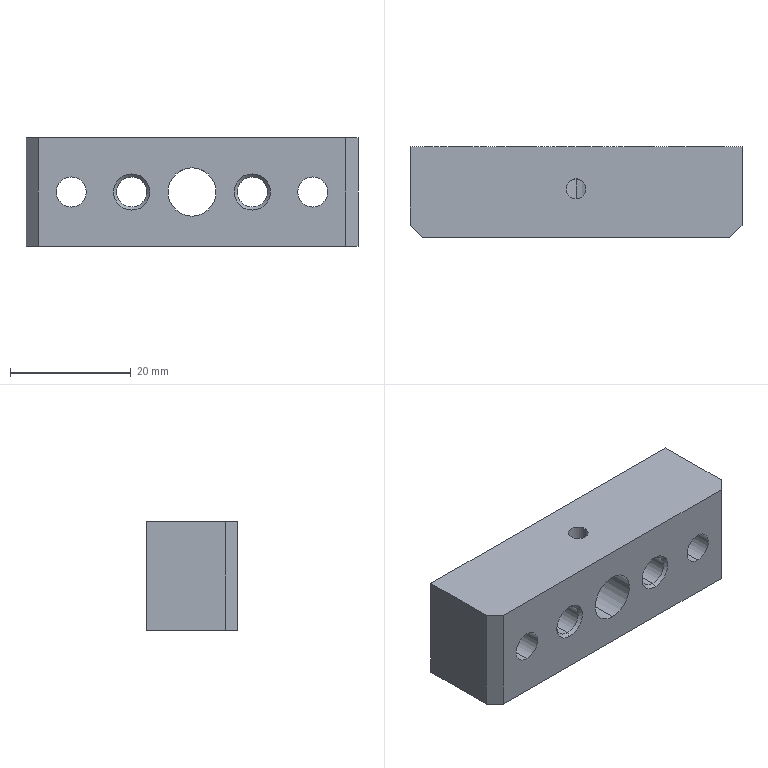Part | SolidWorks | features ICE 9, Chamfer 3, 3DProfileFeature 2, HoleWzd 2, Extrusion 1 | 1 solid | 38 faces | box 55 x 15 x 18 mm | volume 12154 mm3 | cylinder 16 | cone 12 | plane 10 | commonest cylinder face diameters 5 x8 8 x6 3.3 x2
STEP:
#1=CARTESIAN_POINT('',(-20.,14.,-4.));
#2=VERTEX_POINT('',#1);
#3=CARTESIAN_POINT('',(-20.,14.,4.));
#4=VERTEX_POINT('',#3);
#5=CARTESIAN_POINT('',(-20.,14.,0.));
#6=DIRECTION('',(0.,1.,0.));
#7=DIRECTION('',(0.,0.,-1.));
#8=AXIS2_PLACEMENT_3D('',#5,#6,#7);
#9=CIRCLE('',#8,4.);
#10=EDGE_CURVE('',#2,#4,#9,.T.);
#11=ORIENTED_EDGE('',*,*,#10,.F.);
#12=CARTESIAN_POINT('',(-20.,15.,-5.));
#13=VERTEX_POINT('',#12);
#14=CARTESIAN_POINT('',(-20.,14.,-4.));
#15=DIRECTION('',(0.,0.7071,-0.7071));
#16=VECTOR('',#15,1000.);
#17=LINE('',#14,#16);
#18=EDGE_CURVE('',#2,#13,#17,.T.);
#19=ORIENTED_EDGE('',*,*,#18,.T.);
#20=CARTESIAN_POINT('',(-20.,15.,5.));
#21=VERTEX_POINT('',#20);
#22=CARTESIAN_POINT('',(-20.,15.,0.));
#23=DIRECTION('',(0.,-1.,0.));
#24=DIRECTION('',(0.,0.,-1.));
#25=AXIS2_PLACEMENT_3D('',#22,#23,#24);
#26=CIRCLE('',#25,5.);
#27=EDGE_CURVE('',#21,#13,#26,.T.);
#28=ORIENTED_EDGE('',*,*,#27,.F.);
#29=CARTESIAN_POINT('',(-20.,14.,4.));
#30=DIRECTION('',(0.,0.7071,0.7071));
#31=VECTOR('',#30,1000.);
#32=LINE('',#29,#31);
#33=EDGE_CURVE('',#4,#21,#32,.T.);
#34=ORIENTED_EDGE('',*,*,#33,.F.);
#35=EDGE_LOOP('',(#11,#19,#28,#34));
#36=FACE_OUTER_BOUND('',#35,.T.);
#37=CARTESIAN_POINT('',(-20.,14.,0.));
#38=DIRECTION('',(0.,1.,0.));
#39=DIRECTION('',(0.,0.,1.));
#40=AXIS2_PLACEMENT_3D('',#37,#38,#39);
#41=CONICAL_SURFACE('',#40,4.,0.7854);
#42=ADVANCED_FACE('',(#36),#41,.F.);
#43=CARTESIAN_POINT('',(20.,14.,-4.));
#44=VERTEX_POINT('',#43);
#45=CARTESIAN_POINT('',(20.,14.,4.));
#46=VERTEX_POINT('',#45);
#47=CARTESIAN_POINT('',(20.,14.,0.));
#48=DIRECTION('',(0.,1.,0.));
#49=DIRECTION('',(0.,0.,-1.));
#50=AXIS2_PLACEMENT_3D('',#47,#48,#49);
#51=CIRCLE('',#50,4.);
#52=EDGE_CURVE('',#44,#46,#51,.T.);
#53=ORIENTED_EDGE('',*,*,#52,.F.);
#54=CARTESIAN_POINT('',(20.,15.,-5.));
#55=VERTEX_POINT('',#54);
#56=CARTESIAN_POINT('',(20.,14.,-4.));
#57=DIRECTION('',(0.,0.7071,-0.7071));
#58=VECTOR('',#57,1000.);
#59=LINE('',#56,#58);
#60=EDGE_CURVE('',#44,#55,#59,.T.);
#61=ORIENTED_EDGE('',*,*,#60,.T.);
#62=CARTESIAN_POINT('',(20.,15.,5.));
#63=VERTEX_POINT('',#62);
#64=CARTESIAN_POINT('',(20.,15.,0.));
#65=DIRECTION('',(0.,-1.,0.));
#66=DIRECTION('',(0.,0.,-1.));
#67=AXIS2_PLACEMENT_3D('',#64,#65,#66);
#68=CIRCLE('',#67,5.);
#69=EDGE_CURVE('',#63,#55,#68,.T.);
#70=ORIENTED_EDGE('',*,*,#69,.F.);
#71=CARTESIAN_POINT('',(20.,14.,4.));
#72=DIRECTION('',(0.,0.7071,0.7071));
#73=VECTOR('',#72,1000.);
#74=LINE('',#71,#73);
#75=EDGE_CURVE('',#46,#63,#74,.T.);
#76=ORIENTED_EDGE('',*,*,#75,.F.);
#77=EDGE_LOOP('',(#53,#61,#70,#76));
#78=FACE_OUTER_BOUND('',#77,.T.);
#79=CARTESIAN_POINT('',(20.,14.,0.));
#80=DIRECTION('',(0.,1.,0.));
#81=DIRECTION('',(0.,0.,1.));
#82=AXIS2_PLACEMENT_3D('',#79,#80,#81);
#83=CONICAL_SURFACE('',#82,4.,0.7854);
#84=ADVANCED_FACE('',(#78),#83,.F.);
#85=CARTESIAN_POINT('',(-10.,14.5,-2.5));
#86=VERTEX_POINT('',#85);
#87=CARTESIAN_POINT('',(-10.,14.5,2.5));
#88=VERTEX_POINT('',#87);
#89=CARTESIAN_POINT('',(-10.,14.5,0.));
#90=DIRECTION('',(0.,1.,0.));
#91=DIRECTION('',(0.,0.,-1.));
#92=AXIS2_PLACEMENT_3D('',#89,#90,#91);
#93=CIRCLE('',#92,2.5);
#94=EDGE_CURVE('',#86,#88,#93,.T.);
#95=ORIENTED_EDGE('',*,*,#94,.F.);
#96=CARTESIAN_POINT('',(-10.,15.,-3.));
#97=VERTEX_POINT('',#96);
#98=CARTESIAN_POINT('',(-10.,14.5,-2.5));
#99=DIRECTION('',(0.,0.7071,-0.7071));
#100=VECTOR('',#99,1000.);
#101=LINE('',#98,#100);
#102=EDGE_CURVE('',#86,#97,#101,.T.);
#103=ORIENTED_EDGE('',*,*,#102,.T.);
#104=CARTESIAN_POINT('',(-10.,15.,3.));
#105=VERTEX_POINT('',#104);
#106=CARTESIAN_POINT('',(-10.,15.,0.));
#107=DIRECTION('',(0.,-1.,0.));
#108=DIRECTION('',(0.,0.,-1.));
#109=AXIS2_PLACEMENT_3D('',#106,#107,#108);
#110=CIRCLE('',#109,3.);
#111=EDGE_CURVE('',#105,#97,#110,.T.);
#112=ORIENTED_EDGE('',*,*,#111,.F.);
#113=CARTESIAN_POINT('',(-10.,14.5,2.5));
#114=DIRECTION('',(0.,0.7071,0.7071));
#115=VECTOR('',#114,1000.);
#116=LINE('',#113,#115);
#117=EDGE_CURVE('',#88,#105,#116,.T.);
#118=ORIENTED_EDGE('',*,*,#117,.F.);
#119=EDGE_LOOP('',(#95,#103,#112,#118));
#120=FACE_OUTER_BOUND('',#119,.T.);
#121=CARTESIAN_POINT('',(-10.,14.5,0.));
#122=DIRECTION('',(0.,1.,0.));
#123=DIRECTION('',(0.,0.,1.));
#124=AXIS2_PLACEMENT_3D('',#121,#122,#123);
#125=CONICAL_SURFACE('',#124,2.5,0.7854);
#126=ADVANCED_FACE('',(#120),#125,.F.);
#127=CARTESIAN_POINT('',(10.,14.5,-2.5));
#128=VERTEX_POINT('',#127);
#129=CARTESIAN_POINT('',(10.,14.5,2.5));
#130=VERTEX_POINT('',#129);
#131=CARTESIAN_POINT('',(10.,14.5,0.));
#132=DIRECTION('',(0.,1.,0.));
#133=DIRECTION('',(0.,0.,-1.));
#134=AXIS2_PLACEMENT_3D('',#131,#132,#133);
#135=CIRCLE('',#134,2.5);
#136=EDGE_CURVE('',#128,#130,#135,.T.);
#137=ORIENTED_EDGE('',*,*,#136,.F.);
#138=CARTESIAN_POINT('',(10.,15.,-3.));
#139=VERTEX_POINT('',#138);
#140=CARTESIAN_POINT('',(10.,14.5,-2.5));
#141=DIRECTION('',(0.,0.7071,-0.7071));
#142=VECTOR('',#141,1000.);
#143=LINE('',#140,#142);
#144=EDGE_CURVE('',#128,#139,#143,.T.);
#145=ORIENTED_EDGE('',*,*,#144,.T.);
#146=CARTESIAN_POINT('',(10.,15.,3.));
#147=VERTEX_POINT('',#146);
#148=CARTESIAN_POINT('',(10.,15.,0.));
#149=DIRECTION('',(0.,-1.,0.));
#150=DIRECTION('',(0.,0.,-1.));
#151=AXIS2_PLACEMENT_3D('',#148,#149,#150);
#152=CIRCLE('',#151,3.);
#153=EDGE_CURVE('',#147,#139,#152,.T.);
#154=ORIENTED_EDGE('',*,*,#153,.F.);
#155=CARTESIAN_POINT('',(10.,14.5,2.5));
#156=DIRECTION('',(0.,0.7071,0.7071));
#157=VECTOR('',#156,1000.);
#158=LINE('',#155,#157);
#159=EDGE_CURVE('',#130,#147,#158,.T.);
#160=ORIENTED_EDGE('',*,*,#159,.F.);
#161=EDGE_LOOP('',(#137,#145,#154,#160));
#162=FACE_OUTER_BOUND('',#161,.T.);
#163=CARTESIAN_POINT('',(10.,14.5,0.));
#164=DIRECTION('',(0.,1.,0.));
#165=DIRECTION('',(0.,0.,1.));
#166=AXIS2_PLACEMENT_3D('',#163,#164,#165);
#167=CONICAL_SURFACE('',#166,2.5,0.7854);
#168=ADVANCED_FACE('',(#162),#167,.F.);
#169=CARTESIAN_POINT('',(10.,0.5,2.5));
#170=VERTEX_POINT('',#169);
#171=CARTESIAN_POINT('',(10.,0.5,-2.5));
#172=VERTEX_POINT('',#171);
#173=CARTESIAN_POINT('',(10.,0.5,0.));
#174=DIRECTION('',(0.,-1.,0.));
#175=DIRECTION('',(0.,0.,1.));
#176=AXIS2_PLACEMENT_3D('',#173,#174,#175);
#177=CIRCLE('',#176,2.5);
#178=EDGE_CURVE('',#170,#172,#177,.T.);
#179=ORIENTED_EDGE('',*,*,#178,.F.);
#180=CARTESIAN_POINT('',(10.,0.,3.));
#181=VERTEX_POINT('',#180);
#182=CARTESIAN_POINT('',(10.,0.,3.));
#183=DIRECTION('',(0.,-0.7071,0.7071));
#184=VECTOR('',#183,1000.);
#185=LINE('',#182,#184);
#186=EDGE_CURVE('',#170,#181,#185,.T.);
#187=ORIENTED_EDGE('',*,*,#186,.T.);
#188=CARTESIAN_POINT('',(10.,0.,-3.));
#189=VERTEX_POINT('',#188);
#190=CARTESIAN_POINT('',(10.,0.,0.));
#191=DIRECTION('',(0.,1.,0.));
#192=DIRECTION('',(0.,0.,1.));
#193=AXIS2_PLACEMENT_3D('',#190,#191,#192);
#194=CIRCLE('',#193,3.);
#195=EDGE_CURVE('',#189,#181,#194,.T.);
#196=ORIENTED_EDGE('',*,*,#195,.F.);
#197=CARTESIAN_POINT('',(10.,0.,-3.));
#198=DIRECTION('',(0.,-0.7071,-0.7071));
#199=VECTOR('',#198,1000.);
#200=LINE('',#197,#199);
#201=EDGE_CURVE('',#172,#189,#200,.T.);
#202=ORIENTED_EDGE('',*,*,#201,.F.);
#203=EDGE_LOOP('',(#179,#187,#196,#202));
#204=FACE_OUTER_BOUND('',#203,.T.);
#205=CARTESIAN_POINT('',(10.,0.,0.));
#206=DIRECTION('',(0.,-1.,0.));
#207=DIRECTION('',(0.,0.,-1.));
#208=AXIS2_PLACEMENT_3D('',#205,#206,#207);
#209=CONICAL_SURFACE('',#208,3.,0.7854);
#210=ADVANCED_FACE('',(#204),#209,.F.);
#211=CARTESIAN_POINT('',(-10.,0.5,2.5));
#212=VERTEX_POINT('',#211);
#213=CARTESIAN_POINT('',(-10.,0.5,-2.5));
#214=VERTEX_POINT('',#213);
#215=CARTESIAN_POINT('',(-10.,0.5,0.));
#216=DIRECTION('',(0.,-1.,0.));
#217=DIRECTION('',(0.,0.,1.));
#218=AXIS2_PLACEMENT_3D('',#215,#216,#217);
#219=CIRCLE('',#218,2.5);
#220=EDGE_CURVE('',#212,#214,#219,.T.);
#221=ORIENTED_EDGE('',*,*,#220,.F.);
#222=CARTESIAN_POINT('',(-10.,0.,3.));
#223=VERTEX_POINT('',#222);
#224=CARTESIAN_POINT('',(-10.,0.,3.));
#225=DIRECTION('',(0.,-0.7071,0.7071));
#226=VECTOR('',#225,1000.);
#227=LINE('',#224,#226);
#228=EDGE_CURVE('',#212,#223,#227,.T.);
#229=ORIENTED_EDGE('',*,*,#228,.T.);
#230=CARTESIAN_POINT('',(-10.,0.,-3.));
#231=VERTEX_POINT('',#230);
#232=CARTESIAN_POINT('',(-10.,0.,0.));
#233=DIRECTION('',(0.,1.,0.));
#234=DIRECTION('',(0.,0.,1.));
#235=AXIS2_PLACEMENT_3D('',#232,#233,#234);
#236=CIRCLE('',#235,3.);
#237=EDGE_CURVE('',#231,#223,#236,.T.);
#238=ORIENTED_EDGE('',*,*,#237,.F.);
#239=CARTESIAN_POINT('',(-10.,0.,-3.));
#240=DIRECTION('',(0.,-0.7071,-0.7071));
#241=VECTOR('',#240,1000.);
#242=LINE('',#239,#241);
#243=EDGE_CURVE('',#214,#231,#242,.T.);
#244=ORIENTED_EDGE('',*,*,#243,.F.);
#245=EDGE_LOOP('',(#221,#229,#238,#244));
#246=FACE_OUTER_BOUND('',#245,.T.);
#247=CARTESIAN_POINT('',(-10.,0.,0.));
#248=DIRECTION('',(0.,-1.,0.));
#249=DIRECTION('',(0.,0.,-1.));
#250=AXIS2_PLACEMENT_3D('',#247,#248,#249);
#251=CONICAL_SURFACE('',#250,3.,0.7854);
#252=ADVANCED_FACE('',(#246),#251,.F.);
#253=CARTESIAN_POINT('',(-1.65,8.,3.644));
#254=VERTEX_POINT('',#253);
#255=CARTESIAN_POINT('',(0.,6.35,4.));
#256=VERTEX_POINT('',#255);
#257=CARTESIAN_POINT('',(-1.65,8.,3.644));
#258=CARTESIAN_POINT('',(-1.65,7.783,3.644));
#259=CARTESIAN_POINT('',(-1.606,7.564,3.665));
#260=CARTESIAN_POINT('',(-1.481,7.266,3.716));
#261=CARTESIAN_POINT('',(-1.43,7.169,3.736));
#262=CARTESIAN_POINT('',(-1.31,6.992,3.78));
#263=CARTESIAN_POINT('',(-1.243,6.91,3.803));
#264=CARTESIAN_POINT('',(-1.092,6.758,3.849));
#265=CARTESIAN_POINT('',(-1.008,6.689,3.872));
#266=CARTESIAN_POINT('',(-0.831,6.571,3.914));
#267=CARTESIAN_POINT('',(-0.7367,6.52,3.933));
#268=CARTESIAN_POINT('',(-0.4348,6.393,3.982));
#269=CARTESIAN_POINT('',(-0.2205,6.35,4.));
#270=CARTESIAN_POINT('',(0.,6.35,4.));
#271=B_SPLINE_CURVE_WITH_KNOTS('',3,(#257,#258,#259,#260,#261,#262,#263,#264,#265,#266,#267,#268,#269,#270),.UNSPECIFIED.,.F.,.F.,(4,2,2,2,2,2,4),(0.007825,0.008476,0.008802,0.009128,0.009454,0.00978,0.01043),.UNSPECIFIED.);
#272=EDGE_CURVE('',#254,#256,#271,.T.);
#273=ORIENTED_EDGE('',*,*,#272,.F.);
#274=CARTESIAN_POINT('',(-1.65,8.,9.));
#275=VERTEX_POINT('',#274);
#276=CARTESIAN_POINT('',(-1.65,8.,9.));
#277=DIRECTION('',(0.,0.,1.));
#278=VECTOR('',#277,1000.);
#279=LINE('',#276,#278);
#280=EDGE_CURVE('',#254,#275,#279,.T.);
#281=ORIENTED_EDGE('',*,*,#280,.T.);
#282=CARTESIAN_POINT('',(1.65,8.,9.));
#283=VERTEX_POINT('',#282);
#284=CARTESIAN_POINT('',(0.,8.,9.));
#285=DIRECTION('',(0.,0.,1.));
#286=DIRECTION('',(1.,0.,0.));
#287=AXIS2_PLACEMENT_3D('',#284,#285,#286);
#288=CIRCLE('',#287,1.65);
#289=EDGE_CURVE('',#275,#283,#288,.T.);
#290=ORIENTED_EDGE('',*,*,#289,.T.);
#291=CARTESIAN_POINT('',(1.65,8.,3.644));
#292=VERTEX_POINT('',#291);
#293=CARTESIAN_POINT('',(1.65,8.,9.));
#294=DIRECTION('',(0.,0.,1.));
#295=VECTOR('',#294,1000.);
#296=LINE('',#293,#295);
#297=EDGE_CURVE('',#292,#283,#296,.T.);
#298=ORIENTED_EDGE('',*,*,#297,.F.);
#299=CARTESIAN_POINT('',(0.,6.35,4.));
#300=CARTESIAN_POINT('',(0.1104,6.35,4.));
#301=CARTESIAN_POINT('',(0.2187,6.361,3.995));
#302=CARTESIAN_POINT('',(0.4314,6.404,3.978));
#303=CARTESIAN_POINT('',(0.537,6.436,3.965));
#304=CARTESIAN_POINT('',(0.8361,6.561,3.917));
#305=CARTESIAN_POINT('',(1.018,6.684,3.872));
#306=CARTESIAN_POINT('',(1.318,6.985,3.78));
#307=CARTESIAN_POINT('',(1.44,7.167,3.733));
#308=CARTESIAN_POINT('',(1.564,7.464,3.682));
#309=CARTESIAN_POINT('',(1.597,7.569,3.668));
#310=CARTESIAN_POINT('',(1.639,7.783,3.649));
#311=CARTESIAN_POINT('',(1.65,7.891,3.644));
#312=CARTESIAN_POINT('',(1.65,8.,3.644));
#313=B_SPLINE_CURVE_WITH_KNOTS('',3,(#299,#300,#301,#302,#303,#304,#305,#306,#307,#308,#309,#310,#311,#312),.UNSPECIFIED.,.F.,.F.,(4,2,2,2,2,2,4),(0.,0.0003262,0.0006525,0.001305,0.001957,0.002284,0.00261),.UNSPECIFIED.);
#314=EDGE_CURVE('',#256,#292,#313,.T.);
#315=ORIENTED_EDGE('',*,*,#314,.F.);
#316=EDGE_LOOP('',(#273,#281,#290,#298,#315));
#317=FACE_OUTER_BOUND('',#316,.T.);
#318=CARTESIAN_POINT('',(0.,8.,9.));
#319=DIRECTION('',(0.,0.,1.));
#320=DIRECTION('',(1.,0.,0.));
#321=AXIS2_PLACEMENT_3D('',#318,#319,#320);
#322=CYLINDRICAL_SURFACE('',#321,1.65);
#323=ADVANCED_FACE('',(#317),#322,.F.);
#324=ORIENTED_EDGE('',*,*,#178,.T.);
#325=CARTESIAN_POINT('',(10.,-5.,-2.5));
#326=DIRECTION('',(0.,1.,0.));
#327=VECTOR('',#326,1000.);
#328=LINE('',#325,#327);
#329=EDGE_CURVE('',#172,#128,#328,.T.);
#330=ORIENTED_EDGE('',*,*,#329,.T.);
#331=ORIENTED_EDGE('',*,*,#136,.T.);
#332=CARTESIAN_POINT('',(10.,-5.,2.5));
#333=DIRECTION('',(0.,1.,0.));
#334=VECTOR('',#333,1000.);
#335=LINE('',#332,#334);
#336=EDGE_CURVE('',#170,#130,#335,.T.);
#337=ORIENTED_EDGE('',*,*,#336,.F.);
#338=EDGE_LOOP('',(#324,#330,#331,#337));
#339=FACE_OUTER_BOUND('',#338,.T.);
#340=CARTESIAN_POINT('',(10.,-5.,0.));
#341=DIRECTION('',(0.,1.,0.));
#342=DIRECTION('',(0.,0.,1.));
#343=AXIS2_PLACEMENT_3D('',#340,#341,#342);
#344=CYLINDRICAL_SURFACE('',#343,2.5);
#345=ADVANCED_FACE('',(#339),#344,.F.);
#346=ORIENTED_EDGE('',*,*,#220,.T.);
#347=CARTESIAN_POINT('',(-10.,-5.,-2.5));
#348=DIRECTION('',(0.,1.,0.));
#349=VECTOR('',#348,1000.);
#350=LINE('',#347,#349);
#351=EDGE_CURVE('',#214,#86,#350,.T.);
#352=ORIENTED_EDGE('',*,*,#351,.T.);
#353=ORIENTED_EDGE('',*,*,#94,.T.);
#354=CARTESIAN_POINT('',(-10.,-5.,2.5));
#355=DIRECTION('',(0.,1.,0.));
#356=VECTOR('',#355,1000.);
#357=LINE('',#354,#356);
#358=EDGE_CURVE('',#212,#88,#357,.T.);
#359=ORIENTED_EDGE('',*,*,#358,.F.);
#360=EDGE_LOOP('',(#346,#352,#353,#359));
#361=FACE_OUTER_BOUND('',#360,.T.);
#362=CARTESIAN_POINT('',(-10.,-5.,0.));
#363=DIRECTION('',(0.,1.,0.));
#364=DIRECTION('',(0.,0.,1.));
#365=AXIS2_PLACEMENT_3D('',#362,#363,#364);
#366=CYLINDRICAL_SURFACE('',#365,2.5);
#367=ADVANCED_FACE('',(#361),#366,.F.);
#368=CARTESIAN_POINT('',(0.,0.,-4.));
#369=VERTEX_POINT('',#368);
#370=CARTESIAN_POINT('',(0.,0.,4.));
#371=VERTEX_POINT('',#370);
#372=CARTESIAN_POINT('',(0.,0.,0.));
#373=DIRECTION('',(0.,1.,0.));
#374=DIRECTION('',(0.,0.,1.));
#375=AXIS2_PLACEMENT_3D('',#372,#373,#374);
#376=CIRCLE('',#375,4.);
#377=EDGE_CURVE('',#369,#371,#376,.T.);
#378=ORIENTED_EDGE('',*,*,#377,.F.);
#379=CARTESIAN_POINT('',(0.,15.,-4.));
#380=VERTEX_POINT('',#379);
#381=CARTESIAN_POINT('',(0.,20.,-4.));
#382=DIRECTION('',(0.,1.,0.));
#383=VECTOR('',#382,1000.);
#384=LINE('',#381,#383);
#385=EDGE_CURVE('',#369,#380,#384,.T.);
#386=ORIENTED_EDGE('',*,*,#385,.T.);
#387=CARTESIAN_POINT('',(0.,15.,4.));
#388=VERTEX_POINT('',#387);
#389=CARTESIAN_POINT('',(0.,15.,0.));
#390=DIRECTION('',(0.,1.,0.));
#391=DIRECTION('',(0.,0.,-1.));
#392=AXIS2_PLACEMENT_3D('',#389,#390,#391);
#393=CIRCLE('',#392,4.);
#394=EDGE_CURVE('',#380,#388,#393,.T.);
#395=ORIENTED_EDGE('',*,*,#394,.T.);
#396=CARTESIAN_POINT('',(0.,9.65,4.));
#397=VERTEX_POINT('',#396);
#398=CARTESIAN_POINT('',(0.,20.,4.));
#399=DIRECTION('',(0.,1.,0.));
#400=VECTOR('',#399,1000.);
#401=LINE('',#398,#400);
#402=EDGE_CURVE('',#397,#388,#401,.T.);
#403=ORIENTED_EDGE('',*,*,#402,.F.);
#404=CARTESIAN_POINT('',(0.,9.65,4.));
#405=CARTESIAN_POINT('',(-0.1086,9.65,4.));
#406=CARTESIAN_POINT('',(-0.2189,9.639,3.995));
#407=CARTESIAN_POINT('',(-0.4327,9.596,3.978));
#408=CARTESIAN_POINT('',(-0.536,9.564,3.965));
#409=CARTESIAN_POINT('',(-0.8356,9.439,3.917));
#410=CARTESIAN_POINT('',(-1.016,9.318,3.872));
#411=CARTESIAN_POINT('',(-1.244,9.09,3.803));
#412=CARTESIAN_POINT('',(-1.311,9.007,3.78));
#413=CARTESIAN_POINT('',(-1.43,8.83,3.736));
#414=CARTESIAN_POINT('',(-1.482,8.734,3.716));
#415=CARTESIAN_POINT('',(-1.565,8.535,3.682));
#416=CARTESIAN_POINT('',(-1.596,8.432,3.668));
#417=CARTESIAN_POINT('',(-1.639,8.219,3.649));
#418=CARTESIAN_POINT('',(-1.65,8.109,3.644));
#419=CARTESIAN_POINT('',(-1.65,8.,3.644));
#420=B_SPLINE_CURVE_WITH_KNOTS('',3,(#404,#405,#406,#407,#408,#409,#410,#411,#412,#413,#414,#415,#416,#417,#418,#419),.UNSPECIFIED.,.F.,.F.,(4,2,2,2,2,2,2,4),(0.005218,0.005543,0.005869,0.006521,0.006847,0.007173,0.007499,0.007825),.UNSPECIFIED.);
#421=EDGE_CURVE('',#397,#254,#420,.T.);
#422=ORIENTED_EDGE('',*,*,#421,.T.);
#423=ORIENTED_EDGE('',*,*,#272,.T.);
#424=CARTESIAN_POINT('',(0.,20.,4.));
#425=DIRECTION('',(0.,1.,0.));
#426=VECTOR('',#425,1000.);
#427=LINE('',#424,#426);
#428=EDGE_CURVE('',#371,#256,#427,.T.);
#429=ORIENTED_EDGE('',*,*,#428,.F.);
#430=EDGE_LOOP('',(#378,#386,#395,#403,#422,#423,#429));
#431=FACE_OUTER_BOUND('',#430,.T.);
#432=CARTESIAN_POINT('',(0.,20.,0.));
#433=DIRECTION('',(0.,1.,0.));
#434=DIRECTION('',(0.,0.,1.));
#435=AXIS2_PLACEMENT_3D('',#432,#433,#434);
#436=CYLINDRICAL_SURFACE('',#435,4.);
#437=ADVANCED_FACE('',(#431),#436,.F.);
#438=CARTESIAN_POINT('',(20.,0.,-2.5));
#439=VERTEX_POINT('',#438);
#440=CARTESIAN_POINT('',(20.,0.,2.5));
#441=VERTEX_POINT('',#440);
#442=CARTESIAN_POINT('',(20.,0.,0.));
#443=DIRECTION('',(0.,1.,0.));
#444=DIRECTION('',(0.,0.,1.));
#445=AXIS2_PLACEMENT_3D('',#442,#443,#444);
#446=CIRCLE('',#445,2.5);
#447=EDGE_CURVE('',#439,#441,#446,.T.);
#448=ORIENTED_EDGE('',*,*,#447,.F.);
#449=CARTESIAN_POINT('',(20.,5.,-2.5));
#450=VERTEX_POINT('',#449);
#451=CARTESIAN_POINT('',(20.,-8.,-2.5));
#452=DIRECTION('',(0.,1.,0.));
#453=VECTOR('',#452,1000.);
#454=LINE('',#451,#453);
#455=EDGE_CURVE('',#439,#450,#454,.T.);
#456=ORIENTED_EDGE('',*,*,#455,.T.);
#457=CARTESIAN_POINT('',(20.,5.,2.5));
#458=VERTEX_POINT('',#457);
#459=CARTESIAN_POINT('',(20.,5.,0.));
#460=DIRECTION('',(0.,-1.,0.));
#461=DIRECTION('',(0.,0.,-1.));
#462=AXIS2_PLACEMENT_3D('',#459,#460,#461);
#463=CIRCLE('',#462,2.5);
#464=EDGE_CURVE('',#458,#450,#463,.T.);
#465=ORIENTED_EDGE('',*,*,#464,.F.);
#466=CARTESIAN_POINT('',(20.,-8.,2.5));
#467=DIRECTION('',(0.,1.,0.));
#468=VECTOR('',#467,1000.);
#469=LINE('',#466,#468);
#470=EDGE_CURVE('',#441,#458,#469,.T.);
#471=ORIENTED_EDGE('',*,*,#470,.F.);
#472=EDGE_LOOP('',(#448,#456,#465,#471));
#473=FACE_OUTER_BOUND('',#472,.T.);
#474=CARTESIAN_POINT('',(20.,-8.,0.));
#475=DIRECTION('',(0.,1.,0.));
#476=DIRECTION('',(0.,0.,1.));
#477=AXIS2_PLACEMENT_3D('',#474,#475,#476);
#478=CYLINDRICAL_SURFACE('',#477,2.5);
#479=ADVANCED_FACE('',(#473),#478,.F.);
#480=CARTESIAN_POINT('',(-20.,0.,-2.5));
#481=VERTEX_POINT('',#480);
#482=CARTESIAN_POINT('',(-20.,0.,2.5));
#483=VERTEX_POINT('',#482);
#484=CARTESIAN_POINT('',(-20.,0.,0.));
#485=DIRECTION('',(0.,1.,0.));
#486=DIRECTION('',(0.,0.,1.));
#487=AXIS2_PLACEMENT_3D('',#484,#485,#486);
#488=CIRCLE('',#487,2.5);
#489=EDGE_CURVE('',#481,#483,#488,.T.);
#490=ORIENTED_EDGE('',*,*,#489,.F.);
#491=CARTESIAN_POINT('',(-20.,5.,-2.5));
#492=VERTEX_POINT('',#491);
#493=CARTESIAN_POINT('',(-20.,-8.,-2.5));
#494=DIRECTION('',(0.,1.,0.));
#495=VECTOR('',#494,1000.);
#496=LINE('',#493,#495);
#497=EDGE_CURVE('',#481,#492,#496,.T.);
#498=ORIENTED_EDGE('',*,*,#497,.T.);
#499=CARTESIAN_POINT('',(-20.,5.,2.5));
#500=VERTEX_POINT('',#499);
#501=CARTESIAN_POINT('',(-20.,5.,0.));
#502=DIRECTION('',(0.,1.,0.));
#503=DIRECTION('',(0.,0.,1.));
#504=AXIS2_PLACEMENT_3D('',#501,#502,#503);
#505=CIRCLE('',#504,2.5);
#506=EDGE_CURVE('',#492,#500,#505,.T.);
#507=ORIENTED_EDGE('',*,*,#506,.T.);
#508=CARTESIAN_POINT('',(-20.,-8.,2.5));
#509=DIRECTION('',(0.,1.,0.));
#510=VECTOR('',#509,1000.);
#511=LINE('',#508,#510);
#512=EDGE_CURVE('',#483,#500,#511,.T.);
#513=ORIENTED_EDGE('',*,*,#512,.F.);
#514=EDGE_LOOP('',(#490,#498,#507,#513));
#515=FACE_OUTER_BOUND('',#514,.T.);
#516=CARTESIAN_POINT('',(-20.,-8.,0.));
#517=DIRECTION('',(0.,1.,0.));
#518=DIRECTION('',(0.,0.,1.));
#519=AXIS2_PLACEMENT_3D('',#516,#517,#518);
#520=CYLINDRICAL_SURFACE('',#519,2.5);
#521=ADVANCED_FACE('',(#515),#520,.F.);
#522=CARTESIAN_POINT('',(20.,5.,-4.));
#523=VERTEX_POINT('',#522);
#524=CARTESIAN_POINT('',(20.,5.,4.));
#525=VERTEX_POINT('',#524);
#526=CARTESIAN_POINT('',(20.,5.,0.));
#527=DIRECTION('',(0.,1.,0.));
#528=DIRECTION('',(0.,0.,-1.));
#529=AXIS2_PLACEMENT_3D('',#526,#527,#528);
#530=CIRCLE('',#529,4.);
#531=EDGE_CURVE('',#523,#525,#530,.T.);
#532=ORIENTED_EDGE('',*,*,#531,.F.);
#533=CARTESIAN_POINT('',(20.,5.,-4.));
#534=DIRECTION('',(0.,1.,0.));
#535=VECTOR('',#534,1000.);
#536=LINE('',#533,#535);
#537=EDGE_CURVE('',#523,#44,#536,.T.);
#538=ORIENTED_EDGE('',*,*,#537,.T.);
#539=ORIENTED_EDGE('',*,*,#52,.T.);
#540=CARTESIAN_POINT('',(20.,5.,4.));
#541=DIRECTION('',(0.,1.,0.));
#542=VECTOR('',#541,1000.);
#543=LINE('',#540,#542);
#544=EDGE_CURVE('',#525,#46,#543,.T.);
#545=ORIENTED_EDGE('',*,*,#544,.F.);
#546=EDGE_LOOP('',(#532,#538,#539,#545));
#547=FACE_OUTER_BOUND('',#546,.T.);
#548=CARTESIAN_POINT('',(20.,5.,0.));
#549=DIRECTION('',(0.,1.,0.));
#550=DIRECTION('',(0.,0.,1.));
#551=AXIS2_PLACEMENT_3D('',#548,#549,#550);
#552=CYLINDRICAL_SURFACE('',#551,4.);
#553=ADVANCED_FACE('',(#547),#552,.F.);
#554=CARTESIAN_POINT('',(-20.,5.,-4.));
#555=VERTEX_POINT('',#554);
#556=CARTESIAN_POINT('',(-20.,5.,4.));
#557=VERTEX_POINT('',#556);
#558=CARTESIAN_POINT('',(-20.,5.,0.));
#559=DIRECTION('',(0.,1.,0.));
#560=DIRECTION('',(0.,0.,1.));
#561=AXIS2_PLACEMENT_3D('',#558,#559,#560);
#562=CIRCLE('',#561,4.);
#563=EDGE_CURVE('',#555,#557,#562,.T.);
#564=ORIENTED_EDGE('',*,*,#563,.F.);
#565=CARTESIAN_POINT('',(-20.,5.,-4.));
#566=DIRECTION('',(0.,1.,0.));
#567=VECTOR('',#566,1000.);
#568=LINE('',#565,#567);
#569=EDGE_CURVE('',#555,#2,#568,.T.);
#570=ORIENTED_EDGE('',*,*,#569,.T.);
#571=ORIENTED_EDGE('',*,*,#10,.T.);
#572=CARTESIAN_POINT('',(-20.,5.,4.));
#573=DIRECTION('',(0.,1.,0.));
#574=VECTOR('',#573,1000.);
#575=LINE('',#572,#574);
#576=EDGE_CURVE('',#557,#4,#575,.T.);
#577=ORIENTED_EDGE('',*,*,#576,.F.);
#578=EDGE_LOOP('',(#564,#570,#571,#577));
#579=FACE_OUTER_BOUND('',#578,.T.);
#580=CARTESIAN_POINT('',(-20.,5.,0.));
#581=DIRECTION('',(0.,1.,0.));
#582=DIRECTION('',(0.,0.,1.));
#583=AXIS2_PLACEMENT_3D('',#580,#581,#582);
#584=CYLINDRICAL_SURFACE('',#583,4.);
#585=ADVANCED_FACE('',(#579),#584,.F.);
#586=CARTESIAN_POINT('',(27.5,15.,-9.));
#587=VERTEX_POINT('',#586);
#588=CARTESIAN_POINT('',(27.5,2.,-9.));
#589=VERTEX_POINT('',#588);
#590=CARTESIAN_POINT('',(27.5,30.,-9.));
#591=DIRECTION('',(0.,-1.,0.));
#592=VECTOR('',#591,1000.);
#593=LINE('',#590,#592);
#594=EDGE_CURVE('',#587,#589,#593,.T.);
#595=ORIENTED_EDGE('',*,*,#594,.F.);
#596=CARTESIAN_POINT('',(27.5,15.,9.));
#597=VERTEX_POINT('',#596);
#598=CARTESIAN_POINT('',(27.5,15.,-13.));
#599=DIRECTION('',(0.,0.,1.));
#600=VECTOR('',#599,1000.);
#601=LINE('',#598,#600);
#602=EDGE_CURVE('',#587,#597,#601,.T.);
#603=ORIENTED_EDGE('',*,*,#602,.T.);
#604=CARTESIAN_POINT('',(27.5,2.,9.));
#605=VERTEX_POINT('',#604);
#606=CARTESIAN_POINT('',(27.5,30.,9.));
#607=DIRECTION('',(0.,-1.,0.));
#608=VECTOR('',#607,1000.);
#609=LINE('',#606,#608);
#610=EDGE_CURVE('',#597,#605,#609,.T.);
#611=ORIENTED_EDGE('',*,*,#610,.T.);
#612=CARTESIAN_POINT('',(27.5,2.,-9.));
#613=DIRECTION('',(0.,0.,-1.));
#614=VECTOR('',#613,1000.);
#615=LINE('',#612,#614);
#616=EDGE_CURVE('',#605,#589,#615,.T.);
#617=ORIENTED_EDGE('',*,*,#616,.T.);
#618=EDGE_LOOP('',(#595,#603,#611,#617));
#619=FACE_OUTER_BOUND('',#618,.T.);
#620=CARTESIAN_POINT('',(27.5,30.,-9.));
#621=DIRECTION('',(-1.,0.,0.));
#622=DIRECTION('',(0.,0.,1.));
#623=AXIS2_PLACEMENT_3D('',#620,#621,#622);
#624=PLANE('',#623);
#625=ADVANCED_FACE('',(#619),#624,.F.);
#626=CARTESIAN_POINT('',(-27.5,15.,-9.));
#627=VERTEX_POINT('',#626);
#628=CARTESIAN_POINT('',(-27.5,2.,-9.));
#629=VERTEX_POINT('',#628);
#630=CARTESIAN_POINT('',(-27.5,30.,-9.));
#631=DIRECTION('',(0.,-1.,0.));
#632=VECTOR('',#631,1000.);
#633=LINE('',#630,#632);
#634=EDGE_CURVE('',#627,#629,#633,.T.);
#635=ORIENTED_EDGE('',*,*,#634,.F.);
#636=CARTESIAN_POINT('',(-27.5,15.,-9.));
#637=DIRECTION('',(1.,0.,0.));
#638=VECTOR('',#637,1000.);
#639=LINE('',#636,#638);
#640=EDGE_CURVE('',#627,#587,#639,.T.);
#641=ORIENTED_EDGE('',*,*,#640,.T.);
#642=ORIENTED_EDGE('',*,*,#594,.T.);
#643=CARTESIAN_POINT('',(25.5,0.,-9.));
#644=VERTEX_POINT('',#643);
#645=CARTESIAN_POINT('',(27.5,2.,-9.));
#646=DIRECTION('',(-0.7071,-0.7071,0.));
#647=VECTOR('',#646,1000.);
#648=LINE('',#645,#647);
#649=EDGE_CURVE('',#589,#644,#648,.T.);
#650=ORIENTED_EDGE('',*,*,#649,.T.);
#651=CARTESIAN_POINT('',(-25.5,0.,-9.));
#652=VERTEX_POINT('',#651);
#653=CARTESIAN_POINT('',(-27.5,0.,-9.));
#654=DIRECTION('',(-1.,0.,0.));
#655=VECTOR('',#654,1000.);
#656=LINE('',#653,#655);
#657=EDGE_CURVE('',#644,#652,#656,.T.);
#658=ORIENTED_EDGE('',*,*,#657,.T.);
#659=CARTESIAN_POINT('',(-27.5,2.,-9.));
#660=DIRECTION('',(-0.7071,0.7071,0.));
#661=VECTOR('',#660,1000.);
#662=LINE('',#659,#661);
#663=EDGE_CURVE('',#652,#629,#662,.T.);
#664=ORIENTED_EDGE('',*,*,#663,.T.);
#665=EDGE_LOOP('',(#635,#641,#642,#650,#658,#664));
#666=FACE_OUTER_BOUND('',#665,.T.);
#667=CARTESIAN_POINT('',(-27.5,30.,-9.));
#668=DIRECTION('',(0.,0.,1.));
#669=DIRECTION('',(1.,0.,0.));
#670=AXIS2_PLACEMENT_3D('',#667,#668,#669);
#671=PLANE('',#670);
#672=ADVANCED_FACE('',(#666),#671,.F.);
#673=CARTESIAN_POINT('',(-27.5,15.,9.));
#674=VERTEX_POINT('',#673);
#675=CARTESIAN_POINT('',(-27.5,2.,9.));
#676=VERTEX_POINT('',#675);
#677=CARTESIAN_POINT('',(-27.5,30.,9.));
#678=DIRECTION('',(0.,-1.,0.));
#679=VECTOR('',#678,1000.);
#680=LINE('',#677,#679);
#681=EDGE_CURVE('',#674,#676,#680,.T.);
#682=ORIENTED_EDGE('',*,*,#681,.F.);
#683=CARTESIAN_POINT('',(-27.5,15.,-13.));
#684=DIRECTION('',(0.,0.,1.));
#685=VECTOR('',#684,1000.);
#686=LINE('',#683,#685);
#687=EDGE_CURVE('',#627,#674,#686,.T.);
#688=ORIENTED_EDGE('',*,*,#687,.F.);
#689=ORIENTED_EDGE('',*,*,#634,.T.);
#690=CARTESIAN_POINT('',(-27.5,2.,-9.));
#691=DIRECTION('',(0.,0.,1.));
#692=VECTOR('',#691,1000.);
#693=LINE('',#690,#692);
#694=EDGE_CURVE('',#629,#676,#693,.T.);
#695=ORIENTED_EDGE('',*,*,#694,.T.);
#696=EDGE_LOOP('',(#682,#688,#689,#695));
#697=FACE_OUTER_BOUND('',#696,.T.);
#698=CARTESIAN_POINT('',(-27.5,30.,-9.));
#699=DIRECTION('',(1.,0.,0.));
#700=DIRECTION('',(0.,0.,-1.));
#701=AXIS2_PLACEMENT_3D('',#698,#699,#700);
#702=PLANE('',#701);
#703=ADVANCED_FACE('',(#697),#702,.F.);
#704=CARTESIAN_POINT('',(0.,8.,9.));
#705=DIRECTION('',(0.,0.,1.));
#706=DIRECTION('',(1.,0.,0.));
#707=AXIS2_PLACEMENT_3D('',#704,#705,#706);
#708=CIRCLE('',#707,1.65);
#709=EDGE_CURVE('',#283,#275,#708,.T.);
#710=ORIENTED_EDGE('',*,*,#709,.F.);
#711=ORIENTED_EDGE('',*,*,#289,.F.);
#712=EDGE_LOOP('',(#710,#711));
#713=FACE_BOUND('',#712,.T.);
#714=ORIENTED_EDGE('',*,*,#610,.F.);
#715=CARTESIAN_POINT('',(-27.5,15.,9.));
#716=DIRECTION('',(1.,0.,0.));
#717=VECTOR('',#716,1000.);
#718=LINE('',#715,#717);
#719=EDGE_CURVE('',#674,#597,#718,.T.);
#720=ORIENTED_EDGE('',*,*,#719,.F.);
#721=ORIENTED_EDGE('',*,*,#681,.T.);
#722=CARTESIAN_POINT('',(-25.5,0.,9.));
#723=VERTEX_POINT('',#722);
#724=CARTESIAN_POINT('',(-27.5,2.,9.));
#725=DIRECTION('',(0.7071,-0.7071,0.));
#726=VECTOR('',#725,1000.);
#727=LINE('',#724,#726);
#728=EDGE_CURVE('',#676,#723,#727,.T.);
#729=ORIENTED_EDGE('',*,*,#728,.T.);
#730=CARTESIAN_POINT('',(25.5,0.,9.));
#731=VERTEX_POINT('',#730);
#732=CARTESIAN_POINT('',(-27.5,0.,9.));
#733=DIRECTION('',(1.,0.,0.));
#734=VECTOR('',#733,1000.);
#735=LINE('',#732,#734);
#736=EDGE_CURVE('',#723,#731,#735,.T.);
#737=ORIENTED_EDGE('',*,*,#736,.T.);
#738=CARTESIAN_POINT('',(27.5,2.,9.));
#739=DIRECTION('',(0.7071,0.7071,0.));
#740=VECTOR('',#739,1000.);
#741=LINE('',#738,#740);
#742=EDGE_CURVE('',#731,#605,#741,.T.);
#743=ORIENTED_EDGE('',*,*,#742,.T.);
#744=EDGE_LOOP('',(#714,#720,#721,#729,#737,#743));
#745=FACE_OUTER_BOUND('',#744,.T.);
#746=CARTESIAN_POINT('',(-27.5,30.,9.));
#747=DIRECTION('',(0.,0.,-1.));
#748=DIRECTION('',(-1.,0.,0.));
#749=AXIS2_PLACEMENT_3D('',#746,#747,#748);
#750=PLANE('',#749);
#751=ADVANCED_FACE('',(#713,#745),#750,.F.);
#752=ORIENTED_EDGE('',*,*,#237,.T.);
#753=CARTESIAN_POINT('',(-10.,0.,0.));
#754=DIRECTION('',(0.,1.,0.));
#755=DIRECTION('',(0.,0.,1.));
#756=AXIS2_PLACEMENT_3D('',#753,#754,#755);
#757=CIRCLE('',#756,3.);
#758=EDGE_CURVE('',#223,#231,#757,.T.);
#759=ORIENTED_EDGE('',*,*,#758,.T.);
#760=EDGE_LOOP('',(#752,#759));
#761=FACE_BOUND('',#760,.T.);
#762=ORIENTED_EDGE('',*,*,#195,.T.);
#763=CARTESIAN_POINT('',(10.,0.,0.));
#764=DIRECTION('',(0.,1.,0.));
#765=DIRECTION('',(0.,0.,1.));
#766=AXIS2_PLACEMENT_3D('',#763,#764,#765);
#767=CIRCLE('',#766,3.);
#768=EDGE_CURVE('',#181,#189,#767,.T.);
#769=ORIENTED_EDGE('',*,*,#768,.T.);
#770=EDGE_LOOP('',(#762,#769));
#771=FACE_BOUND('',#770,.T.);
#772=CARTESIAN_POINT('',(0.,0.,0.));
#773=DIRECTION('',(0.,1.,0.));
#774=DIRECTION('',(0.,0.,1.));
#775=AXIS2_PLACEMENT_3D('',#772,#773,#774);
#776=CIRCLE('',#775,4.);
#777=EDGE_CURVE('',#371,#369,#776,.T.);
#778=ORIENTED_EDGE('',*,*,#777,.T.);
#779=ORIENTED_EDGE('',*,*,#377,.T.);
#780=EDGE_LOOP('',(#778,#779));
#781=FACE_BOUND('',#780,.T.);
#782=CARTESIAN_POINT('',(20.,0.,0.));
#783=DIRECTION('',(0.,1.,0.));
#784=DIRECTION('',(0.,0.,1.));
#785=AXIS2_PLACEMENT_3D('',#782,#783,#784);
#786=CIRCLE('',#785,2.5);
#787=EDGE_CURVE('',#441,#439,#786,.T.);
#788=ORIENTED_EDGE('',*,*,#787,.T.);
#789=ORIENTED_EDGE('',*,*,#447,.T.);
#790=EDGE_LOOP('',(#788,#789));
#791=FACE_BOUND('',#790,.T.);
#792=CARTESIAN_POINT('',(-20.,0.,0.));
#793=DIRECTION('',(0.,1.,0.));
#794=DIRECTION('',(0.,0.,1.));
#795=AXIS2_PLACEMENT_3D('',#792,#793,#794);
#796=CIRCLE('',#795,2.5);
#797=EDGE_CURVE('',#483,#481,#796,.T.);
#798=ORIENTED_EDGE('',*,*,#797,.T.);
#799=ORIENTED_EDGE('',*,*,#489,.T.);
#800=EDGE_LOOP('',(#798,#799));
#801=FACE_BOUND('',#800,.T.);
#802=ORIENTED_EDGE('',*,*,#657,.F.);
#803=CARTESIAN_POINT('',(25.5,0.,0.));
#804=DIRECTION('',(0.,0.,1.));
#805=VECTOR('',#804,1000.);
#806=LINE('',#803,#805);
#807=EDGE_CURVE('',#644,#731,#806,.T.);
#808=ORIENTED_EDGE('',*,*,#807,.T.);
#809=ORIENTED_EDGE('',*,*,#736,.F.);
#810=CARTESIAN_POINT('',(-25.5,0.,0.));
#811=DIRECTION('',(0.,0.,-1.));
#812=VECTOR('',#811,1000.);
#813=LINE('',#810,#812);
#814=EDGE_CURVE('',#723,#652,#813,.T.);
#815=ORIENTED_EDGE('',*,*,#814,.T.);
#816=EDGE_LOOP('',(#802,#808,#809,#815));
#817=FACE_OUTER_BOUND('',#816,.T.);
#818=CARTESIAN_POINT('',(0.,0.,0.));
#819=DIRECTION('',(0.,1.,0.));
#820=DIRECTION('',(0.,0.,1.));
#821=AXIS2_PLACEMENT_3D('',#818,#819,#820);
#822=PLANE('',#821);
#823=ADVANCED_FACE('',(#761,#771,#781,#791,#801,#817),#822,.F.);
#824=ORIENTED_EDGE('',*,*,#569,.F.);
#825=CARTESIAN_POINT('',(-20.,5.,0.));
#826=DIRECTION('',(0.,1.,0.));
#827=DIRECTION('',(0.,0.,1.));
#828=AXIS2_PLACEMENT_3D('',#825,#826,#827);
#829=CIRCLE('',#828,4.);
#830=EDGE_CURVE('',#557,#555,#829,.T.);
#831=ORIENTED_EDGE('',*,*,#830,.F.);
#832=ORIENTED_EDGE('',*,*,#576,.T.);
#833=CARTESIAN_POINT('',(-20.,14.,0.));
#834=DIRECTION('',(0.,1.,0.));
#835=DIRECTION('',(0.,0.,-1.));
#836=AXIS2_PLACEMENT_3D('',#833,#834,#835);
#837=CIRCLE('',#836,4.);
#838=EDGE_CURVE('',#4,#2,#837,.T.);
#839=ORIENTED_EDGE('',*,*,#838,.T.);
#840=EDGE_LOOP('',(#824,#831,#832,#839));
#841=FACE_OUTER_BOUND('',#840,.T.);
#842=CARTESIAN_POINT('',(-20.,5.,0.));
#843=DIRECTION('',(0.,1.,0.));
#844=DIRECTION('',(0.,0.,1.));
#845=AXIS2_PLACEMENT_3D('',#842,#843,#844);
#846=CYLINDRICAL_SURFACE('',#845,4.);
#847=ADVANCED_FACE('',(#841),#846,.F.);
#848=CARTESIAN_POINT('',(-20.,5.,0.));
#849=DIRECTION('',(0.,1.,0.));
#850=DIRECTION('',(0.,0.,1.));
#851=AXIS2_PLACEMENT_3D('',#848,#849,#850);
#852=CIRCLE('',#851,2.5);
#853=EDGE_CURVE('',#500,#492,#852,.T.);
#854=ORIENTED_EDGE('',*,*,#853,.F.);
#855=ORIENTED_EDGE('',*,*,#506,.F.);
#856=EDGE_LOOP('',(#854,#855));
#857=FACE_BOUND('',#856,.T.);
#858=ORIENTED_EDGE('',*,*,#830,.T.);
#859=ORIENTED_EDGE('',*,*,#563,.T.);
#860=EDGE_LOOP('',(#858,#859));
#861=FACE_OUTER_BOUND('',#860,.T.);
#862=CARTESIAN_POINT('',(-20.,5.,0.));
#863=DIRECTION('',(0.,1.,0.));
#864=DIRECTION('',(0.,0.,1.));
#865=AXIS2_PLACEMENT_3D('',#862,#863,#864);
#866=PLANE('',#865);
#867=ADVANCED_FACE('',(#857,#861),#866,.T.);
#868=ORIENTED_EDGE('',*,*,#537,.F.);
#869=CARTESIAN_POINT('',(20.,5.,0.));
#870=DIRECTION('',(0.,1.,0.));
#871=DIRECTION('',(0.,0.,-1.));
#872=AXIS2_PLACEMENT_3D('',#869,#870,#871);
#873=CIRCLE('',#872,4.);
#874=EDGE_CURVE('',#525,#523,#873,.T.);
#875=ORIENTED_EDGE('',*,*,#874,.F.);
#876=ORIENTED_EDGE('',*,*,#544,.T.);
#877=CARTESIAN_POINT('',(20.,14.,0.));
#878=DIRECTION('',(0.,1.,0.));
#879=DIRECTION('',(0.,0.,-1.));
#880=AXIS2_PLACEMENT_3D('',#877,#878,#879);
#881=CIRCLE('',#880,4.);
#882=EDGE_CURVE('',#46,#44,#881,.T.);
#883=ORIENTED_EDGE('',*,*,#882,.T.);
#884=EDGE_LOOP('',(#868,#875,#876,#883));
#885=FACE_OUTER_BOUND('',#884,.T.);
#886=CARTESIAN_POINT('',(20.,5.,0.));
#887=DIRECTION('',(0.,1.,0.));
#888=DIRECTION('',(0.,0.,1.));
#889=AXIS2_PLACEMENT_3D('',#886,#887,#888);
#890=CYLINDRICAL_SURFACE('',#889,4.);
#891=ADVANCED_FACE('',(#885),#890,.F.);
#892=ORIENTED_EDGE('',*,*,#464,.T.);
#893=CARTESIAN_POINT('',(20.,5.,0.));
#894=DIRECTION('',(0.,-1.,0.));
#895=DIRECTION('',(0.,0.,-1.));
#896=AXIS2_PLACEMENT_3D('',#893,#894,#895);
#897=CIRCLE('',#896,2.5);
#898=EDGE_CURVE('',#450,#458,#897,.T.);
#899=ORIENTED_EDGE('',*,*,#898,.T.);
#900=EDGE_LOOP('',(#892,#899));
#901=FACE_BOUND('',#900,.T.);
#902=ORIENTED_EDGE('',*,*,#874,.T.);
#903=ORIENTED_EDGE('',*,*,#531,.T.);
#904=EDGE_LOOP('',(#902,#903));
#905=FACE_OUTER_BOUND('',#904,.T.);
#906=CARTESIAN_POINT('',(20.,5.,0.));
#907=DIRECTION('',(0.,-1.,0.));
#908=DIRECTION('',(0.,0.,-1.));
#909=AXIS2_PLACEMENT_3D('',#906,#907,#908);
#910=PLANE('',#909);
#911=ADVANCED_FACE('',(#901,#905),#910,.F.);
#912=ORIENTED_EDGE('',*,*,#497,.F.);
#913=ORIENTED_EDGE('',*,*,#797,.F.);
#914=ORIENTED_EDGE('',*,*,#512,.T.);
#915=ORIENTED_EDGE('',*,*,#853,.T.);
#916=EDGE_LOOP('',(#912,#913,#914,#915));
#917=FACE_OUTER_BOUND('',#916,.T.);
#918=CARTESIAN_POINT('',(-20.,-8.,0.));
#919=DIRECTION('',(0.,1.,0.));
#920=DIRECTION('',(0.,0.,1.));
#921=AXIS2_PLACEMENT_3D('',#918,#919,#920);
#922=CYLINDRICAL_SURFACE('',#921,2.5);
#923=ADVANCED_FACE('',(#917),#922,.F.);
#924=ORIENTED_EDGE('',*,*,#455,.F.);
#925=ORIENTED_EDGE('',*,*,#787,.F.);
#926=ORIENTED_EDGE('',*,*,#470,.T.);
#927=ORIENTED_EDGE('',*,*,#898,.F.);
#928=EDGE_LOOP('',(#924,#925,#926,#927));
#929=FACE_OUTER_BOUND('',#928,.T.);
#930=CARTESIAN_POINT('',(20.,-8.,0.));
#931=DIRECTION('',(0.,1.,0.));
#932=DIRECTION('',(0.,0.,1.));
#933=AXIS2_PLACEMENT_3D('',#930,#931,#932);
#934=CYLINDRICAL_SURFACE('',#933,2.5);
#935=ADVANCED_FACE('',(#929),#934,.F.);
#936=ORIENTED_EDGE('',*,*,#385,.F.);
#937=ORIENTED_EDGE('',*,*,#777,.F.);
#938=ORIENTED_EDGE('',*,*,#428,.T.);
#939=ORIENTED_EDGE('',*,*,#314,.T.);
#940=CARTESIAN_POINT('',(1.65,8.,3.644));
#941=CARTESIAN_POINT('',(1.65,8.109,3.644));
#942=CARTESIAN_POINT('',(1.639,8.22,3.649));
#943=CARTESIAN_POINT('',(1.596,8.432,3.668));
#944=CARTESIAN_POINT('',(1.564,8.536,3.682));
#945=CARTESIAN_POINT('',(1.48,8.737,3.716));
#946=CARTESIAN_POINT('',(1.429,8.831,3.736));
#947=CARTESIAN_POINT('',(1.31,9.008,3.78));
#948=CARTESIAN_POINT('',(1.241,9.092,3.803));
#949=CARTESIAN_POINT('',(1.091,9.243,3.849));
#950=CARTESIAN_POINT('',(1.008,9.31,3.872));
#951=CARTESIAN_POINT('',(0.8301,9.43,3.914));
#952=CARTESIAN_POINT('',(0.7341,9.482,3.933));
#953=CARTESIAN_POINT('',(0.4367,9.606,3.981));
#954=CARTESIAN_POINT('',(0.2173,9.65,4.));
#955=CARTESIAN_POINT('',(0.,9.65,4.));
#956=B_SPLINE_CURVE_WITH_KNOTS('',3,(#940,#941,#942,#943,#944,#945,#946,#947,#948,#949,#950,#951,#952,#953,#954,#955),.UNSPECIFIED.,.F.,.F.,(4,2,2,2,2,2,2,4),(0.00261,0.002936,0.003262,0.003588,0.003914,0.00424,0.004566,0.005218),.UNSPECIFIED.);
#957=EDGE_CURVE('',#292,#397,#956,.T.);
#958=ORIENTED_EDGE('',*,*,#957,.T.);
#959=ORIENTED_EDGE('',*,*,#402,.T.);
#960=CARTESIAN_POINT('',(0.,15.,0.));
#961=DIRECTION('',(0.,1.,0.));
#962=DIRECTION('',(0.,0.,-1.));
#963=AXIS2_PLACEMENT_3D('',#960,#961,#962);
#964=CIRCLE('',#963,4.);
#965=EDGE_CURVE('',#388,#380,#964,.T.);
#966=ORIENTED_EDGE('',*,*,#965,.T.);
#967=EDGE_LOOP('',(#936,#937,#938,#939,#958,#959,#966));
#968=FACE_OUTER_BOUND('',#967,.T.);
#969=CARTESIAN_POINT('',(0.,20.,0.));
#970=DIRECTION('',(0.,1.,0.));
#971=DIRECTION('',(0.,0.,1.));
#972=AXIS2_PLACEMENT_3D('',#969,#970,#971);
#973=CYLINDRICAL_SURFACE('',#972,4.);
#974=ADVANCED_FACE('',(#968),#973,.F.);
#975=ORIENTED_EDGE('',*,*,#742,.F.);
#976=ORIENTED_EDGE('',*,*,#807,.F.);
#977=ORIENTED_EDGE('',*,*,#649,.F.);
#978=ORIENTED_EDGE('',*,*,#616,.F.);
#979=EDGE_LOOP('',(#975,#976,#977,#978));
#980=FACE_OUTER_BOUND('',#979,.T.);
#981=CARTESIAN_POINT('',(27.5,2.,-9.));
#982=DIRECTION('',(-0.7071,0.7071,0.));
#983=DIRECTION('',(0.,0.,-1.));
#984=AXIS2_PLACEMENT_3D('',#981,#982,#983);
#985=PLANE('',#984);
#986=ADVANCED_FACE('',(#980),#985,.F.);
#987=ORIENTED_EDGE('',*,*,#663,.F.);
#988=ORIENTED_EDGE('',*,*,#814,.F.);
#989=ORIENTED_EDGE('',*,*,#728,.F.);
#990=ORIENTED_EDGE('',*,*,#694,.F.);
#991=EDGE_LOOP('',(#987,#988,#989,#990));
#992=FACE_OUTER_BOUND('',#991,.T.);
#993=CARTESIAN_POINT('',(-27.5,2.,-9.));
#994=DIRECTION('',(0.7071,0.7071,0.));
#995=DIRECTION('',(0.,0.,1.));
#996=AXIS2_PLACEMENT_3D('',#993,#994,#995);
#997=PLANE('',#996);
#998=ADVANCED_FACE('',(#992),#997,.F.);
#999=ORIENTED_EDGE('',*,*,#351,.F.);
#1000=CARTESIAN_POINT('',(-10.,0.5,0.));
#1001=DIRECTION('',(0.,-1.,0.));
#1002=DIRECTION('',(0.,0.,1.));
#1003=AXIS2_PLACEMENT_3D('',#1000,#1001,#1002);
#1004=CIRCLE('',#1003,2.5);
#1005=EDGE_CURVE('',#214,#212,#1004,.T.);
#1006=ORIENTED_EDGE('',*,*,#1005,.T.);
#1007=ORIENTED_EDGE('',*,*,#358,.T.);
#1008=CARTESIAN_POINT('',(-10.,14.5,0.));
#1009=DIRECTION('',(0.,1.,0.));
#1010=DIRECTION('',(0.,0.,-1.));
#1011=AXIS2_PLACEMENT_3D('',#1008,#1009,#1010);
#1012=CIRCLE('',#1011,2.5);
#1013=EDGE_CURVE('',#88,#86,#1012,.T.);
#1014=ORIENTED_EDGE('',*,*,#1013,.T.);
#1015=EDGE_LOOP('',(#999,#1006,#1007,#1014));
#1016=FACE_OUTER_BOUND('',#1015,.T.);
#1017=CARTESIAN_POINT('',(-10.,-5.,0.));
#1018=DIRECTION('',(0.,1.,0.));
#1019=DIRECTION('',(0.,0.,1.));
#1020=AXIS2_PLACEMENT_3D('',#1017,#1018,#1019);
#1021=CYLINDRICAL_SURFACE('',#1020,2.5);
#1022=ADVANCED_FACE('',(#1016),#1021,.F.);
#1023=ORIENTED_EDGE('',*,*,#329,.F.);
#1024=CARTESIAN_POINT('',(10.,0.5,0.));
#1025=DIRECTION('',(0.,-1.,0.));
#1026=DIRECTION('',(0.,0.,1.));
#1027=AXIS2_PLACEMENT_3D('',#1024,#1025,#1026);
#1028=CIRCLE('',#1027,2.5);
#1029=EDGE_CURVE('',#172,#170,#1028,.T.);
#1030=ORIENTED_EDGE('',*,*,#1029,.T.);
#1031=ORIENTED_EDGE('',*,*,#336,.T.);
#1032=CARTESIAN_POINT('',(10.,14.5,0.));
#1033=DIRECTION('',(0.,1.,0.));
#1034=DIRECTION('',(0.,0.,-1.));
#1035=AXIS2_PLACEMENT_3D('',#1032,#1033,#1034);
#1036=CIRCLE('',#1035,2.5);
#1037=EDGE_CURVE('',#130,#128,#1036,.T.);
#1038=ORIENTED_EDGE('',*,*,#1037,.T.);
#1039=EDGE_LOOP('',(#1023,#1030,#1031,#1038));
#1040=FACE_OUTER_BOUND('',#1039,.T.);
#1041=CARTESIAN_POINT('',(10.,-5.,0.));
#1042=DIRECTION('',(0.,1.,0.));
#1043=DIRECTION('',(0.,0.,1.));
#1044=AXIS2_PLACEMENT_3D('',#1041,#1042,#1043);
#1045=CYLINDRICAL_SURFACE('',#1044,2.5);
#1046=ADVANCED_FACE('',(#1040),#1045,.F.);
#1047=ORIENTED_EDGE('',*,*,#280,.F.);
#1048=ORIENTED_EDGE('',*,*,#421,.F.);
#1049=ORIENTED_EDGE('',*,*,#957,.F.);
#1050=ORIENTED_EDGE('',*,*,#297,.T.);
#1051=ORIENTED_EDGE('',*,*,#709,.T.);
#1052=EDGE_LOOP('',(#1047,#1048,#1049,#1050,#1051));
#1053=FACE_OUTER_BOUND('',#1052,.T.);
#1054=CARTESIAN_POINT('',(0.,8.,9.));
#1055=DIRECTION('',(0.,0.,1.));
#1056=DIRECTION('',(1.,0.,0.));
#1057=AXIS2_PLACEMENT_3D('',#1054,#1055,#1056);
#1058=CYLINDRICAL_SURFACE('',#1057,1.65);
#1059=ADVANCED_FACE('',(#1053),#1058,.F.);
#1060=ORIENTED_EDGE('',*,*,#69,.T.);
#1061=CARTESIAN_POINT('',(20.,15.,0.));
#1062=DIRECTION('',(0.,-1.,0.));
#1063=DIRECTION('',(0.,0.,-1.));
#1064=AXIS2_PLACEMENT_3D('',#1061,#1062,#1063);
#1065=CIRCLE('',#1064,5.);
#1066=EDGE_CURVE('',#55,#63,#1065,.T.);
#1067=ORIENTED_EDGE('',*,*,#1066,.T.);
#1068=EDGE_LOOP('',(#1060,#1067));
#1069=FACE_BOUND('',#1068,.T.);
#1070=ORIENTED_EDGE('',*,*,#27,.T.);
#1071=CARTESIAN_POINT('',(-20.,15.,0.));
#1072=DIRECTION('',(0.,-1.,0.));
#1073=DIRECTION('',(0.,0.,-1.));
#1074=AXIS2_PLACEMENT_3D('',#1071,#1072,#1073);
#1075=CIRCLE('',#1074,5.);
#1076=EDGE_CURVE('',#13,#21,#1075,.T.);
#1077=ORIENTED_EDGE('',*,*,#1076,.T.);
#1078=EDGE_LOOP('',(#1070,#1077));
#1079=FACE_BOUND('',#1078,.T.);
#1080=ORIENTED_EDGE('',*,*,#153,.T.);
#1081=CARTESIAN_POINT('',(10.,15.,0.));
#1082=DIRECTION('',(0.,-1.,0.));
#1083=DIRECTION('',(0.,0.,-1.));
#1084=AXIS2_PLACEMENT_3D('',#1081,#1082,#1083);
#1085=CIRCLE('',#1084,3.);
#1086=EDGE_CURVE('',#139,#147,#1085,.T.);
#1087=ORIENTED_EDGE('',*,*,#1086,.T.);
#1088=EDGE_LOOP('',(#1080,#1087));
#1089=FACE_BOUND('',#1088,.T.);
#1090=ORIENTED_EDGE('',*,*,#111,.T.);
#1091=CARTESIAN_POINT('',(-10.,15.,0.));
#1092=DIRECTION('',(0.,-1.,0.));
#1093=DIRECTION('',(0.,0.,-1.));
#1094=AXIS2_PLACEMENT_3D('',#1091,#1092,#1093);
#1095=CIRCLE('',#1094,3.);
#1096=EDGE_CURVE('',#97,#105,#1095,.T.);
#1097=ORIENTED_EDGE('',*,*,#1096,.T.);
#1098=EDGE_LOOP('',(#1090,#1097));
#1099=FACE_BOUND('',#1098,.T.);
#1100=ORIENTED_EDGE('',*,*,#965,.F.);
#1101=ORIENTED_EDGE('',*,*,#394,.F.);
#1102=EDGE_LOOP('',(#1100,#1101));
#1103=FACE_BOUND('',#1102,.T.);
#1104=ORIENTED_EDGE('',*,*,#687,.T.);
#1105=ORIENTED_EDGE('',*,*,#719,.T.);
#1106=ORIENTED_EDGE('',*,*,#602,.F.);
#1107=ORIENTED_EDGE('',*,*,#640,.F.);
#1108=EDGE_LOOP('',(#1104,#1105,#1106,#1107));
#1109=FACE_OUTER_BOUND('',#1108,.T.);
#1110=CARTESIAN_POINT('',(-27.5,15.,-13.));
#1111=DIRECTION('',(0.,-1.,0.));
#1112=DIRECTION('',(0.,0.,-1.));
#1113=AXIS2_PLACEMENT_3D('',#1110,#1111,#1112);
#1114=PLANE('',#1113);
#1115=ADVANCED_FACE('',(#1069,#1079,#1089,#1099,#1103,#1109),#1114,.F.);
#1116=ORIENTED_EDGE('',*,*,#228,.F.);
#1117=ORIENTED_EDGE('',*,*,#1005,.F.);
#1118=ORIENTED_EDGE('',*,*,#243,.T.);
#1119=ORIENTED_EDGE('',*,*,#758,.F.);
#1120=EDGE_LOOP('',(#1116,#1117,#1118,#1119));
#1121=FACE_OUTER_BOUND('',#1120,.T.);
#1122=CARTESIAN_POINT('',(-10.,0.,0.));
#1123=DIRECTION('',(0.,-1.,0.));
#1124=DIRECTION('',(0.,0.,-1.));
#1125=AXIS2_PLACEMENT_3D('',#1122,#1123,#1124);
#1126=CONICAL_SURFACE('',#1125,3.,0.7854);
#1127=ADVANCED_FACE('',(#1121),#1126,.F.);
#1128=ORIENTED_EDGE('',*,*,#186,.F.);
#1129=ORIENTED_EDGE('',*,*,#1029,.F.);
#1130=ORIENTED_EDGE('',*,*,#201,.T.);
#1131=ORIENTED_EDGE('',*,*,#768,.F.);
#1132=EDGE_LOOP('',(#1128,#1129,#1130,#1131));
#1133=FACE_OUTER_BOUND('',#1132,.T.);
#1134=CARTESIAN_POINT('',(10.,0.,0.));
#1135=DIRECTION('',(0.,-1.,0.));
#1136=DIRECTION('',(0.,0.,-1.));
#1137=AXIS2_PLACEMENT_3D('',#1134,#1135,#1136);
#1138=CONICAL_SURFACE('',#1137,3.,0.7854);
#1139=ADVANCED_FACE('',(#1133),#1138,.F.);
#1140=ORIENTED_EDGE('',*,*,#144,.F.);
#1141=ORIENTED_EDGE('',*,*,#1037,.F.);
#1142=ORIENTED_EDGE('',*,*,#159,.T.);
#1143=ORIENTED_EDGE('',*,*,#1086,.F.);
#1144=EDGE_LOOP('',(#1140,#1141,#1142,#1143));
#1145=FACE_OUTER_BOUND('',#1144,.T.);
#1146=CARTESIAN_POINT('',(10.,14.5,0.));
#1147=DIRECTION('',(0.,1.,0.));
#1148=DIRECTION('',(0.,0.,1.));
#1149=AXIS2_PLACEMENT_3D('',#1146,#1147,#1148);
#1150=CONICAL_SURFACE('',#1149,2.5,0.7854);
#1151=ADVANCED_FACE('',(#1145),#1150,.F.);
#1152=ORIENTED_EDGE('',*,*,#102,.F.);
#1153=ORIENTED_EDGE('',*,*,#1013,.F.);
#1154=ORIENTED_EDGE('',*,*,#117,.T.);
#1155=ORIENTED_EDGE('',*,*,#1096,.F.);
#1156=EDGE_LOOP('',(#1152,#1153,#1154,#1155));
#1157=FACE_OUTER_BOUND('',#1156,.T.);
#1158=CARTESIAN_POINT('',(-10.,14.5,0.));
#1159=DIRECTION('',(0.,1.,0.));
#1160=DIRECTION('',(0.,0.,1.));
#1161=AXIS2_PLACEMENT_3D('',#1158,#1159,#1160);
#1162=CONICAL_SURFACE('',#1161,2.5,0.7854);
#1163=ADVANCED_FACE('',(#1157),#1162,.F.);
#1164=ORIENTED_EDGE('',*,*,#60,.F.);
#1165=ORIENTED_EDGE('',*,*,#882,.F.);
#1166=ORIENTED_EDGE('',*,*,#75,.T.);
#1167=ORIENTED_EDGE('',*,*,#1066,.F.);
#1168=EDGE_LOOP('',(#1164,#1165,#1166,#1167));
#1169=FACE_OUTER_BOUND('',#1168,.T.);
#1170=CARTESIAN_POINT('',(20.,14.,0.));
#1171=DIRECTION('',(0.,1.,0.));
#1172=DIRECTION('',(0.,0.,1.));
#1173=AXIS2_PLACEMENT_3D('',#1170,#1171,#1172);
#1174=CONICAL_SURFACE('',#1173,4.,0.7854);
#1175=ADVANCED_FACE('',(#1169),#1174,.F.);
#1176=ORIENTED_EDGE('',*,*,#18,.F.);
#1177=ORIENTED_EDGE('',*,*,#838,.F.);
#1178=ORIENTED_EDGE('',*,*,#33,.T.);
#1179=ORIENTED_EDGE('',*,*,#1076,.F.);
#1180=EDGE_LOOP('',(#1176,#1177,#1178,#1179));
#1181=FACE_OUTER_BOUND('',#1180,.T.);
#1182=CARTESIAN_POINT('',(-20.,14.,0.));
#1183=DIRECTION('',(0.,1.,0.));
#1184=DIRECTION('',(0.,0.,1.));
#1185=AXIS2_PLACEMENT_3D('',#1182,#1183,#1184);
#1186=CONICAL_SURFACE('',#1185,4.,0.7854);
#1187=ADVANCED_FACE('',(#1181),#1186,.F.);
#1188=CLOSED_SHELL('',(#42,#84,#126,#168,#210,#252,#323,#345,#367,#437,#479,#521,#553,#585,#625,#672,#703,#751,#823,#847,#867,#891,#911,#923,#935,#974,#986,#998,#1022,#1046,#1059,#1115,#1127,#1139,#1151,#1163,#1175,#1187));
#1189=MANIFOLD_SOLID_BREP('',#1188);
#1190=CARTESIAN_POINT('',(0.,0.,0.));
#1191=DIRECTION('',(0.,0.,1.));
#1192=DIRECTION('',(1.,0.,0.));
#1193=AXIS2_PLACEMENT_3D('',#1190,#1191,#1192);
#1194=(LENGTH_UNIT()NAMED_UNIT(*)SI_UNIT(.MILLI.,.METRE.));
#1195=UNCERTAINTY_MEASURE_WITH_UNIT(LENGTH_MEASURE(0.00001),#1194,'','');
#1196=(NAMED_UNIT(*)PLANE_ANGLE_UNIT()SI_UNIT($,.RADIAN.));
#1197=(NAMED_UNIT(*)SI_UNIT($,.STERADIAN.)SOLID_ANGLE_UNIT());
#1198=(GEOMETRIC_REPRESENTATION_CONTEXT(3)GLOBAL_UNCERTAINTY_ASSIGNED_CONTEXT((#1195))GLOBAL_UNIT_ASSIGNED_CONTEXT((#1194,#1196,#1197))REPRESENTATION_CONTEXT('',''));
#1199=ADVANCED_BREP_SHAPE_REPRESENTATION('',(#1189,#1193),#1198);